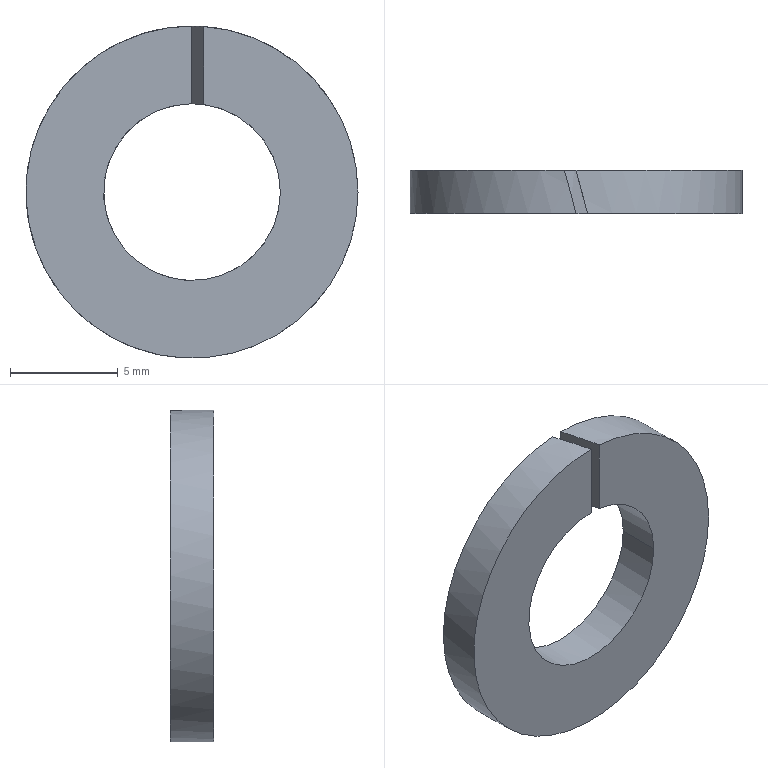Part | STEP file | ZZ24-M8 | 1 solid | 8 faces | box 15.4 x 2 x 15.4 mm | volume 263.048 mm3 | plane 4 | cylinder 4 | commonest cylinder face diameters 8.2 x2 15.4 x2
STEP:
#1=CARTESIAN_POINT('',(0.,0.,0.));
#2=DIRECTION('',(0.,0.,1.));
#3=DIRECTION('',(1.,0.,0.));
#4=AXIS2_PLACEMENT_3D('',#1,#2,#3);
#5=CARTESIAN_POINT('',(0.,0.,7.7));
#6=VERTEX_POINT('',#5);
#7=CARTESIAN_POINT('',(7.7,0.,0.));
#8=VERTEX_POINT('',#7);
#9=CARTESIAN_POINT('',(0.,0.,0.));
#10=DIRECTION('',(0.,-1.,0.));
#11=DIRECTION('',(0.,0.,1.));
#12=AXIS2_PLACEMENT_3D('',#9,#10,#11);
#13=CIRCLE('',#12,7.7);
#14=CARTESIAN_POINT('',(-16.334,0.,16.334));
#15=DIRECTION('',(0.,1.,0.));
#16=DIRECTION('',(1.,0.,0.));
#17=AXIS2_PLACEMENT_3D('',#14,#15,#16);
#18=PLANE('',#17);
#19=CARTESIAN_POINT('',(16.334,8.634));
#20=CARTESIAN_POINT('',(2.997,8.634));
#21=CARTESIAN_POINT('',(9.666,20.184));
#22=CARTESIAN_POINT('',(16.334,31.734));
#23=CARTESIAN_POINT('',(23.003,20.184));
#24=CARTESIAN_POINT('',(29.671,8.634));
#25=CARTESIAN_POINT('',(16.334,8.634));
#26=(BOUNDED_CURVE()B_SPLINE_CURVE(2,(#19,#20,#21,#22,#23,#24,#25),.UNSPECIFIED.,.T.,.F.)B_SPLINE_CURVE_WITH_KNOTS((1,2,2,2,2,1),(-2.094,0.,2.094,4.189,6.283,8.378),.UNSPECIFIED.)CURVE()GEOMETRIC_REPRESENTATION_ITEM()RATIONAL_B_SPLINE_CURVE((1.,0.5,1.,0.5,1.,0.5,1.))REPRESENTATION_ITEM(''));
#27=(GEOMETRIC_REPRESENTATION_CONTEXT(2)PARAMETRIC_REPRESENTATION_CONTEXT()REPRESENTATION_CONTEXT('',''));
#28=DEFINITIONAL_REPRESENTATION('',(#26),#27);
#29=PCURVE('',#18,#28);
#30=CARTESIAN_POINT('',(0.,1.,0.));
#31=DIRECTION('',(0.,1.,0.));
#32=DIRECTION('',(1.,0.,0.));
#33=AXIS2_PLACEMENT_3D('',#30,#31,#32);
#34=CYLINDRICAL_SURFACE('',#33,7.7);
#35=CARTESIAN_POINT('',(4.712,-1.));
#36=DIRECTION('',(-1.,0.));
#37=VECTOR('',#36,1.);
#38=LINE('',#35,#37);
#39=(GEOMETRIC_REPRESENTATION_CONTEXT(2)PARAMETRIC_REPRESENTATION_CONTEXT()REPRESENTATION_CONTEXT('',''));
#40=DEFINITIONAL_REPRESENTATION('',(#38),#39);
#41=PCURVE('',#34,#40);
#42=SURFACE_CURVE('',#13,(#29,#41),.PCURVE_S1.);
#43=EDGE_CURVE('',#6,#8,#42,.T.);
#44=ORIENTED_EDGE('',*,*,#43,.T.);
#45=CARTESIAN_POINT('',(0.5359,0.,7.681));
#46=VERTEX_POINT('',#45);
#47=CARTESIAN_POINT('',(0.,0.,0.));
#48=DIRECTION('',(0.,1.,0.));
#49=DIRECTION('',(0.0696,0.,0.9976));
#50=AXIS2_PLACEMENT_3D('',#47,#48,#49);
#51=CIRCLE('',#50,7.7);
#52=CARTESIAN_POINT('',(16.334,16.334));
#53=DIRECTION('',(0.0696,-0.9976));
#54=AXIS2_PLACEMENT_2D('',#52,#53);
#55=CIRCLE('',#54,7.7);
#56=(GEOMETRIC_REPRESENTATION_CONTEXT(2)PARAMETRIC_REPRESENTATION_CONTEXT()REPRESENTATION_CONTEXT('',''));
#57=DEFINITIONAL_REPRESENTATION('',(#55),#56);
#58=PCURVE('',#18,#57);
#59=CARTESIAN_POINT('',(0.,1.,0.));
#60=DIRECTION('',(0.,1.,0.));
#61=DIRECTION('',(1.,0.,0.));
#62=AXIS2_PLACEMENT_3D('',#59,#60,#61);
#63=CYLINDRICAL_SURFACE('',#62,7.7);
#64=CARTESIAN_POINT('',(4.782,-1.));
#65=DIRECTION('',(1.,0.));
#66=VECTOR('',#65,1.);
#67=LINE('',#64,#66);
#68=(GEOMETRIC_REPRESENTATION_CONTEXT(2)PARAMETRIC_REPRESENTATION_CONTEXT()REPRESENTATION_CONTEXT('',''));
#69=DEFINITIONAL_REPRESENTATION('',(#67),#68);
#70=PCURVE('',#63,#69);
#71=SURFACE_CURVE('',#51,(#58,#70),.PCURVE_S1.);
#72=EDGE_CURVE('',#46,#8,#71,.T.);
#73=ORIENTED_EDGE('',*,*,#72,.F.);
#74=CARTESIAN_POINT('',(0.5359,0.,4.065));
#75=VERTEX_POINT('',#74);
#76=CARTESIAN_POINT('',(0.5359,0.,7.681));
#77=DIRECTION('',(0.,0.,-1.));
#78=VECTOR('',#77,1.);
#79=LINE('',#76,#78);
#80=CARTESIAN_POINT('',(16.87,8.653));
#81=DIRECTION('',(0.,1.));
#82=VECTOR('',#81,1.);
#83=LINE('',#80,#82);
#84=(GEOMETRIC_REPRESENTATION_CONTEXT(2)PARAMETRIC_REPRESENTATION_CONTEXT()REPRESENTATION_CONTEXT('',''));
#85=DEFINITIONAL_REPRESENTATION('',(#83),#84);
#86=PCURVE('',#18,#85);
#87=CARTESIAN_POINT('',(1.08,-2.031,2.745));
#88=DIRECTION('',(0.9659,0.2588,0.));
#89=DIRECTION('',(-0.2588,0.9659,0.));
#90=AXIS2_PLACEMENT_3D('',#87,#88,#89);
#91=PLANE('',#90);
#92=CARTESIAN_POINT('',(2.102,4.937));
#93=DIRECTION('',(0.,-1.));
#94=VECTOR('',#93,1.);
#95=LINE('',#92,#94);
#96=(GEOMETRIC_REPRESENTATION_CONTEXT(2)PARAMETRIC_REPRESENTATION_CONTEXT()REPRESENTATION_CONTEXT('',''));
#97=DEFINITIONAL_REPRESENTATION('',(#95),#96);
#98=PCURVE('',#91,#97);
#99=SURFACE_CURVE('',#79,(#86,#98),.PCURVE_S1.);
#100=EDGE_CURVE('',#46,#75,#99,.T.);
#101=ORIENTED_EDGE('',*,*,#100,.T.);
#102=CARTESIAN_POINT('',(4.1,0.,0.));
#103=VERTEX_POINT('',#102);
#104=CARTESIAN_POINT('',(0.,0.,0.));
#105=DIRECTION('',(0.,-1.,0.));
#106=DIRECTION('',(1.,0.,0.));
#107=AXIS2_PLACEMENT_3D('',#104,#105,#106);
#108=CIRCLE('',#107,4.1);
#109=CARTESIAN_POINT('',(20.434,16.334));
#110=CARTESIAN_POINT('',(20.434,9.233));
#111=CARTESIAN_POINT('',(14.284,12.783));
#112=CARTESIAN_POINT('',(8.134,16.334));
#113=CARTESIAN_POINT('',(14.284,19.885));
#114=CARTESIAN_POINT('',(20.434,23.436));
#115=CARTESIAN_POINT('',(20.434,16.334));
#116=(BOUNDED_CURVE()B_SPLINE_CURVE(2,(#109,#110,#111,#112,#113,#114,#115),.UNSPECIFIED.,.T.,.F.)B_SPLINE_CURVE_WITH_KNOTS((1,2,2,2,2,1),(-2.094,0.,2.094,4.189,6.283,8.378),.UNSPECIFIED.)CURVE()GEOMETRIC_REPRESENTATION_ITEM()RATIONAL_B_SPLINE_CURVE((1.,0.5,1.,0.5,1.,0.5,1.))REPRESENTATION_ITEM(''));
#117=(GEOMETRIC_REPRESENTATION_CONTEXT(2)PARAMETRIC_REPRESENTATION_CONTEXT()REPRESENTATION_CONTEXT('',''));
#118=DEFINITIONAL_REPRESENTATION('',(#116),#117);
#119=PCURVE('',#18,#118);
#120=CARTESIAN_POINT('',(0.,1.,0.));
#121=DIRECTION('',(0.,1.,0.));
#122=DIRECTION('',(1.,0.,0.));
#123=AXIS2_PLACEMENT_3D('',#120,#121,#122);
#124=CYLINDRICAL_SURFACE('',#123,4.1);
#125=CARTESIAN_POINT('',(6.283,-1.));
#126=DIRECTION('',(-1.,0.));
#127=VECTOR('',#126,1.);
#128=LINE('',#125,#127);
#129=(GEOMETRIC_REPRESENTATION_CONTEXT(2)PARAMETRIC_REPRESENTATION_CONTEXT()REPRESENTATION_CONTEXT('',''));
#130=DEFINITIONAL_REPRESENTATION('',(#128),#129);
#131=PCURVE('',#124,#130);
#132=SURFACE_CURVE('',#108,(#119,#131),.PCURVE_S1.);
#133=EDGE_CURVE('',#103,#75,#132,.T.);
#134=ORIENTED_EDGE('',*,*,#133,.F.);
#135=CARTESIAN_POINT('',(0.,0.,4.1));
#136=VERTEX_POINT('',#135);
#137=CARTESIAN_POINT('',(0.,0.,0.));
#138=DIRECTION('',(0.,1.,0.));
#139=DIRECTION('',(1.,0.,0.));
#140=AXIS2_PLACEMENT_3D('',#137,#138,#139);
#141=CIRCLE('',#140,4.1);
#142=CARTESIAN_POINT('',(16.334,16.334));
#143=DIRECTION('',(1.,0.));
#144=AXIS2_PLACEMENT_2D('',#142,#143);
#145=CIRCLE('',#144,4.1);
#146=(GEOMETRIC_REPRESENTATION_CONTEXT(2)PARAMETRIC_REPRESENTATION_CONTEXT()REPRESENTATION_CONTEXT('',''));
#147=DEFINITIONAL_REPRESENTATION('',(#145),#146);
#148=PCURVE('',#18,#147);
#149=CARTESIAN_POINT('',(0.,1.,0.));
#150=DIRECTION('',(0.,1.,0.));
#151=DIRECTION('',(1.,0.,0.));
#152=AXIS2_PLACEMENT_3D('',#149,#150,#151);
#153=CYLINDRICAL_SURFACE('',#152,4.1);
#154=CARTESIAN_POINT('',(0.,-1.));
#155=DIRECTION('',(1.,0.));
#156=VECTOR('',#155,1.);
#157=LINE('',#154,#156);
#158=(GEOMETRIC_REPRESENTATION_CONTEXT(2)PARAMETRIC_REPRESENTATION_CONTEXT()REPRESENTATION_CONTEXT('',''));
#159=DEFINITIONAL_REPRESENTATION('',(#157),#158);
#160=PCURVE('',#153,#159);
#161=SURFACE_CURVE('',#141,(#148,#160),.PCURVE_S1.);
#162=EDGE_CURVE('',#103,#136,#161,.T.);
#163=ORIENTED_EDGE('',*,*,#162,.T.);
#164=CARTESIAN_POINT('',(0.,0.,7.7));
#165=DIRECTION('',(0.,0.,-1.));
#166=VECTOR('',#165,1.);
#167=LINE('',#164,#166);
#168=CARTESIAN_POINT('',(16.334,8.634));
#169=DIRECTION('',(0.,1.));
#170=VECTOR('',#169,1.);
#171=LINE('',#168,#170);
#172=(GEOMETRIC_REPRESENTATION_CONTEXT(2)PARAMETRIC_REPRESENTATION_CONTEXT()REPRESENTATION_CONTEXT('',''));
#173=DEFINITIONAL_REPRESENTATION('',(#171),#172);
#174=PCURVE('',#18,#173);
#175=CARTESIAN_POINT('',(-1.08,4.031,2.745));
#176=DIRECTION('',(-0.9659,-0.2588,0.));
#177=DIRECTION('',(0.2588,-0.9659,0.));
#178=AXIS2_PLACEMENT_3D('',#175,#176,#177);
#179=PLANE('',#178);
#180=CARTESIAN_POINT('',(4.173,4.955));
#181=DIRECTION('',(0.,-1.));
#182=VECTOR('',#181,1.);
#183=LINE('',#180,#182);
#184=(GEOMETRIC_REPRESENTATION_CONTEXT(2)PARAMETRIC_REPRESENTATION_CONTEXT()REPRESENTATION_CONTEXT('',''));
#185=DEFINITIONAL_REPRESENTATION('',(#183),#184);
#186=PCURVE('',#179,#185);
#187=SURFACE_CURVE('',#167,(#174,#186),.PCURVE_S1.);
#188=EDGE_CURVE('',#6,#136,#187,.T.);
#189=ORIENTED_EDGE('',*,*,#188,.F.);
#190=EDGE_LOOP('',(#44,#73,#101,#134,#163,#189));
#191=FACE_BOUND('',#190,.T.);
#192=ADVANCED_FACE('',(#191),#18,.F.);
#193=ORIENTED_EDGE('',*,*,#188,.T.);
#194=CARTESIAN_POINT('',(-0.5359,2.,4.065));
#195=VERTEX_POINT('',#194);
#196=CARTESIAN_POINT('',(-0.5359,2.,4.065));
#197=CARTESIAN_POINT('',(-0.3573,1.334,4.088));
#198=CARTESIAN_POINT('',(-0.1787,0.6668,4.1));
#199=CARTESIAN_POINT('',(0.,0.,4.1));
#200=B_SPLINE_CURVE_WITH_KNOTS('',3,(#196,#197,#198,#199),.UNSPECIFIED.,.F.,.F.,(4,4),(0.,1.),.PIECEWISE_BEZIER_KNOTS.);
#201=CARTESIAN_POINT('',(2.102,1.32));
#202=CARTESIAN_POINT('',(2.792,1.344));
#203=CARTESIAN_POINT('',(3.483,1.355));
#204=CARTESIAN_POINT('',(4.173,1.355));
#205=B_SPLINE_CURVE_WITH_KNOTS('',3,(#201,#202,#203,#204),.UNSPECIFIED.,.F.,.F.,(4,4),(0.,1.),.PIECEWISE_BEZIER_KNOTS.);
#206=(GEOMETRIC_REPRESENTATION_CONTEXT(2)PARAMETRIC_REPRESENTATION_CONTEXT()REPRESENTATION_CONTEXT('',''));
#207=DEFINITIONAL_REPRESENTATION('',(#205),#206);
#208=PCURVE('',#179,#207);
#209=CARTESIAN_POINT('',(4.581,1.));
#210=CARTESIAN_POINT('',(4.583,0.9697));
#211=CARTESIAN_POINT('',(4.587,0.9091));
#212=CARTESIAN_POINT('',(4.593,0.8182));
#213=CARTESIAN_POINT('',(4.599,0.7274));
#214=CARTESIAN_POINT('',(4.605,0.6365));
#215=CARTESIAN_POINT('',(4.611,0.5456));
#216=CARTESIAN_POINT('',(4.617,0.4547));
#217=CARTESIAN_POINT('',(4.623,0.3638));
#218=CARTESIAN_POINT('',(4.629,0.2729));
#219=CARTESIAN_POINT('',(4.635,0.182));
#220=CARTESIAN_POINT('',(4.641,0.09106));
#221=CARTESIAN_POINT('',(4.647,0.0001454));
#222=CARTESIAN_POINT('',(4.653,-0.09077));
#223=CARTESIAN_POINT('',(4.659,-0.1817));
#224=CARTESIAN_POINT('',(4.665,-0.2726));
#225=CARTESIAN_POINT('',(4.671,-0.3635));
#226=CARTESIAN_POINT('',(4.677,-0.4544));
#227=CARTESIAN_POINT('',(4.683,-0.5454));
#228=CARTESIAN_POINT('',(4.689,-0.6363));
#229=CARTESIAN_POINT('',(4.695,-0.7272));
#230=CARTESIAN_POINT('',(4.701,-0.8181));
#231=CARTESIAN_POINT('',(4.706,-0.9091));
#232=CARTESIAN_POINT('',(4.71,-0.9697));
#233=CARTESIAN_POINT('',(4.712,-1.));
#234=B_SPLINE_CURVE_WITH_KNOTS('',3,(#209,#210,#211,#212,#213,#214,#215,#216,#217,#218,#219,#220,#221,#222,#223,#224,#225,#226,#227,#228,#229,#230,#231,#232,#233),.UNSPECIFIED.,.F.,.F.,(4,1,1,1,1,1,1,1,1,1,1,1,1,1,1,1,1,1,1,1,1,1,4),(0.,0.04545,0.09091,0.1364,0.1818,0.2273,0.2727,0.3182,0.3636,0.4091,0.4545,0.5,0.5455,0.5909,0.6364,0.6818,0.7273,0.7727,0.8182,0.8636,0.9091,0.9545,1.),.QUASI_UNIFORM_KNOTS.);
#235=(GEOMETRIC_REPRESENTATION_CONTEXT(2)PARAMETRIC_REPRESENTATION_CONTEXT()REPRESENTATION_CONTEXT('',''));
#236=DEFINITIONAL_REPRESENTATION('',(#234),#235);
#237=PCURVE('',#153,#236);
#238=SURFACE_CURVE('',#200,(#208,#237),.PCURVE_S1.);
#239=EDGE_CURVE('',#195,#136,#238,.T.);
#240=ORIENTED_EDGE('',*,*,#239,.F.);
#241=CARTESIAN_POINT('',(-0.5359,2.,7.681));
#242=VERTEX_POINT('',#241);
#243=CARTESIAN_POINT('',(-0.5359,2.,7.681));
#244=DIRECTION('',(0.,0.,-1.));
#245=VECTOR('',#244,1.);
#246=LINE('',#243,#245);
#247=CARTESIAN_POINT('',(2.102,4.937));
#248=DIRECTION('',(0.,-1.));
#249=VECTOR('',#248,1.);
#250=LINE('',#247,#249);
#251=(GEOMETRIC_REPRESENTATION_CONTEXT(2)PARAMETRIC_REPRESENTATION_CONTEXT()REPRESENTATION_CONTEXT('',''));
#252=DEFINITIONAL_REPRESENTATION('',(#250),#251);
#253=PCURVE('',#179,#252);
#254=CARTESIAN_POINT('',(-16.777,2.,16.52));
#255=DIRECTION('',(0.,1.,0.));
#256=DIRECTION('',(1.,0.,0.));
#257=AXIS2_PLACEMENT_3D('',#254,#255,#256);
#258=PLANE('',#257);
#259=CARTESIAN_POINT('',(16.241,8.839));
#260=DIRECTION('',(0.,1.));
#261=VECTOR('',#260,1.);
#262=LINE('',#259,#261);
#263=(GEOMETRIC_REPRESENTATION_CONTEXT(2)PARAMETRIC_REPRESENTATION_CONTEXT()REPRESENTATION_CONTEXT('',''));
#264=DEFINITIONAL_REPRESENTATION('',(#262),#263);
#265=PCURVE('',#258,#264);
#266=SURFACE_CURVE('',#246,(#253,#265),.PCURVE_S1.);
#267=EDGE_CURVE('',#242,#195,#266,.T.);
#268=ORIENTED_EDGE('',*,*,#267,.F.);
#269=CARTESIAN_POINT('',(-0.0003089,0.001153,-106.985));
#270=DIRECTION('',(0.9659,0.2588,0.));
#271=DIRECTION('',(-0.00467,0.01743,0.9998));
#272=AXIS2_PLACEMENT_3D('',#269,#270,#271);
#273=CIRCLE('',#272,114.685);
#274=CARTESIAN_POINT('',(2.102,4.937));
#275=CARTESIAN_POINT('',(200.71,8.521));
#276=CARTESIAN_POINT('',(104.51,-165.271));
#277=CARTESIAN_POINT('',(8.31,-339.062));
#278=CARTESIAN_POINT('',(-94.097,-168.855));
#279=CARTESIAN_POINT('',(-196.505,1.352));
#280=CARTESIAN_POINT('',(2.102,4.937));
#281=(BOUNDED_CURVE()B_SPLINE_CURVE(2,(#274,#275,#276,#277,#278,#279,#280),.UNSPECIFIED.,.T.,.F.)B_SPLINE_CURVE_WITH_KNOTS((1,2,2,2,2,1),(-2.094,0.,2.094,4.189,6.283,8.378),.UNSPECIFIED.)CURVE()GEOMETRIC_REPRESENTATION_ITEM()RATIONAL_B_SPLINE_CURVE((1.,0.5,1.,0.5,1.,0.5,1.))REPRESENTATION_ITEM(''));
#282=(GEOMETRIC_REPRESENTATION_CONTEXT(2)PARAMETRIC_REPRESENTATION_CONTEXT()REPRESENTATION_CONTEXT('',''));
#283=DEFINITIONAL_REPRESENTATION('',(#281),#282);
#284=PCURVE('',#179,#283);
#285=CARTESIAN_POINT('',(4.643,1.));
#286=CARTESIAN_POINT('',(4.644,0.9697));
#287=CARTESIAN_POINT('',(4.646,0.9091));
#288=CARTESIAN_POINT('',(4.649,0.8182));
#289=CARTESIAN_POINT('',(4.652,0.7273));
#290=CARTESIAN_POINT('',(4.655,0.6364));
#291=CARTESIAN_POINT('',(4.659,0.5455));
#292=CARTESIAN_POINT('',(4.662,0.4546));
#293=CARTESIAN_POINT('',(4.665,0.3637));
#294=CARTESIAN_POINT('',(4.668,0.2728));
#295=CARTESIAN_POINT('',(4.671,0.1819));
#296=CARTESIAN_POINT('',(4.674,0.09095));
#297=CARTESIAN_POINT('',(4.678,0.00004082));
#298=CARTESIAN_POINT('',(4.681,-0.09087));
#299=CARTESIAN_POINT('',(4.684,-0.1818));
#300=CARTESIAN_POINT('',(4.687,-0.2727));
#301=CARTESIAN_POINT('',(4.69,-0.3636));
#302=CARTESIAN_POINT('',(4.693,-0.4545));
#303=CARTESIAN_POINT('',(4.697,-0.5454));
#304=CARTESIAN_POINT('',(4.7,-0.6363));
#305=CARTESIAN_POINT('',(4.703,-0.7273));
#306=CARTESIAN_POINT('',(4.706,-0.8182));
#307=CARTESIAN_POINT('',(4.709,-0.9091));
#308=CARTESIAN_POINT('',(4.711,-0.9697));
#309=CARTESIAN_POINT('',(4.712,-1.));
#310=B_SPLINE_CURVE_WITH_KNOTS('',3,(#285,#286,#287,#288,#289,#290,#291,#292,#293,#294,#295,#296,#297,#298,#299,#300,#301,#302,#303,#304,#305,#306,#307,#308,#309),.UNSPECIFIED.,.F.,.F.,(4,1,1,1,1,1,1,1,1,1,1,1,1,1,1,1,1,1,1,1,1,1,4),(0.,0.0008207,0.001641,0.002462,0.003283,0.004103,0.004924,0.005745,0.006566,0.007386,0.008207,0.009028,0.009848,0.01067,0.01149,0.01231,0.01313,0.01395,0.01477,0.01559,0.01641,0.01723,0.01806),.QUASI_UNIFORM_KNOTS.);
#311=(GEOMETRIC_REPRESENTATION_CONTEXT(2)PARAMETRIC_REPRESENTATION_CONTEXT()REPRESENTATION_CONTEXT('',''));
#312=DEFINITIONAL_REPRESENTATION('',(#310),#311);
#313=PCURVE('',#34,#312);
#314=SURFACE_CURVE('',#273,(#284,#313),.PCURVE_S1.);
#315=EDGE_CURVE('',#242,#6,#314,.T.);
#316=ORIENTED_EDGE('',*,*,#315,.T.);
#317=EDGE_LOOP('',(#193,#240,#268,#316));
#318=FACE_BOUND('',#317,.T.);
#319=ADVANCED_FACE('',(#318),#179,.F.);
#320=CARTESIAN_POINT('',(7.7,2.,0.));
#321=VERTEX_POINT('',#320);
#322=CARTESIAN_POINT('',(7.7,0.,0.));
#323=DIRECTION('',(0.,1.,0.));
#324=VECTOR('',#323,1.);
#325=LINE('',#322,#324);
#326=CARTESIAN_POINT('',(0.,-1.));
#327=DIRECTION('',(0.,1.));
#328=VECTOR('',#327,1.);
#329=LINE('',#326,#328);
#330=(GEOMETRIC_REPRESENTATION_CONTEXT(2)PARAMETRIC_REPRESENTATION_CONTEXT()REPRESENTATION_CONTEXT('',''));
#331=DEFINITIONAL_REPRESENTATION('',(#329),#330);
#332=PCURVE('',#34,#331);
#333=CARTESIAN_POINT('',(6.283,-1.));
#334=DIRECTION('',(0.,1.));
#335=VECTOR('',#334,1.);
#336=LINE('',#333,#335);
#337=(GEOMETRIC_REPRESENTATION_CONTEXT(2)PARAMETRIC_REPRESENTATION_CONTEXT()REPRESENTATION_CONTEXT('',''));
#338=DEFINITIONAL_REPRESENTATION('',(#336),#337);
#339=PCURVE('',#63,#338);
#340=SURFACE_CURVE('',#325,(#332,#339),.PCURVE_S1.);
#341=EDGE_CURVE('',#8,#321,#340,.T.);
#342=ORIENTED_EDGE('',*,*,#341,.F.);
#343=ORIENTED_EDGE('',*,*,#43,.F.);
#344=ORIENTED_EDGE('',*,*,#315,.F.);
#345=CARTESIAN_POINT('',(0.,2.,0.));
#346=DIRECTION('',(0.,1.,0.));
#347=DIRECTION('',(1.,0.,0.));
#348=AXIS2_PLACEMENT_3D('',#345,#346,#347);
#349=CIRCLE('',#348,7.7);
#350=CARTESIAN_POINT('',(0.,1.));
#351=DIRECTION('',(1.,0.));
#352=VECTOR('',#351,1.);
#353=LINE('',#350,#352);
#354=(GEOMETRIC_REPRESENTATION_CONTEXT(2)PARAMETRIC_REPRESENTATION_CONTEXT()REPRESENTATION_CONTEXT('',''));
#355=DEFINITIONAL_REPRESENTATION('',(#353),#354);
#356=PCURVE('',#34,#355);
#357=CARTESIAN_POINT('',(16.777,16.52));
#358=DIRECTION('',(1.,0.));
#359=AXIS2_PLACEMENT_2D('',#357,#358);
#360=CIRCLE('',#359,7.7);
#361=(GEOMETRIC_REPRESENTATION_CONTEXT(2)PARAMETRIC_REPRESENTATION_CONTEXT()REPRESENTATION_CONTEXT('',''));
#362=DEFINITIONAL_REPRESENTATION('',(#360),#361);
#363=PCURVE('',#258,#362);
#364=SURFACE_CURVE('',#349,(#356,#363),.PCURVE_S1.);
#365=EDGE_CURVE('',#321,#242,#364,.T.);
#366=ORIENTED_EDGE('',*,*,#365,.F.);
#367=EDGE_LOOP('',(#342,#343,#344,#366));
#368=FACE_BOUND('',#367,.T.);
#369=ADVANCED_FACE('',(#368),#34,.T.);
#370=CARTESIAN_POINT('',(4.1,2.,0.));
#371=VERTEX_POINT('',#370);
#372=CARTESIAN_POINT('',(0.,2.,0.));
#373=DIRECTION('',(0.,-1.,0.));
#374=DIRECTION('',(-0.1307,0.,0.9914));
#375=AXIS2_PLACEMENT_3D('',#372,#373,#374);
#376=CIRCLE('',#375,4.1);
#377=CARTESIAN_POINT('',(16.241,12.456));
#378=CARTESIAN_POINT('',(9.201,13.384));
#379=CARTESIAN_POINT('',(13.525,19.017));
#380=CARTESIAN_POINT('',(17.849,24.65));
#381=CARTESIAN_POINT('',(20.565,18.089));
#382=CARTESIAN_POINT('',(23.282,11.527));
#383=CARTESIAN_POINT('',(16.241,12.456));
#384=(BOUNDED_CURVE()B_SPLINE_CURVE(2,(#377,#378,#379,#380,#381,#382,#383),.UNSPECIFIED.,.T.,.F.)B_SPLINE_CURVE_WITH_KNOTS((1,2,2,2,2,1),(-2.094,0.,2.094,4.189,6.283,8.378),.UNSPECIFIED.)CURVE()GEOMETRIC_REPRESENTATION_ITEM()RATIONAL_B_SPLINE_CURVE((1.,0.5,1.,0.5,1.,0.5,1.))REPRESENTATION_ITEM(''));
#385=(GEOMETRIC_REPRESENTATION_CONTEXT(2)PARAMETRIC_REPRESENTATION_CONTEXT()REPRESENTATION_CONTEXT('',''));
#386=DEFINITIONAL_REPRESENTATION('',(#384),#385);
#387=PCURVE('',#258,#386);
#388=CARTESIAN_POINT('',(4.581,1.));
#389=DIRECTION('',(-1.,0.));
#390=VECTOR('',#389,1.);
#391=LINE('',#388,#390);
#392=(GEOMETRIC_REPRESENTATION_CONTEXT(2)PARAMETRIC_REPRESENTATION_CONTEXT()REPRESENTATION_CONTEXT('',''));
#393=DEFINITIONAL_REPRESENTATION('',(#391),#392);
#394=PCURVE('',#153,#393);
#395=SURFACE_CURVE('',#376,(#387,#394),.PCURVE_S1.);
#396=EDGE_CURVE('',#195,#371,#395,.T.);
#397=ORIENTED_EDGE('',*,*,#396,.T.);
#398=CARTESIAN_POINT('',(0.,2.,4.1));
#399=VERTEX_POINT('',#398);
#400=CARTESIAN_POINT('',(0.,2.,0.));
#401=DIRECTION('',(0.,-1.,0.));
#402=DIRECTION('',(1.,0.,0.));
#403=AXIS2_PLACEMENT_3D('',#400,#401,#402);
#404=CIRCLE('',#403,4.1);
#405=CARTESIAN_POINT('',(20.877,16.52));
#406=CARTESIAN_POINT('',(20.877,9.419));
#407=CARTESIAN_POINT('',(14.727,12.97));
#408=CARTESIAN_POINT('',(8.577,16.52));
#409=CARTESIAN_POINT('',(14.727,20.071));
#410=CARTESIAN_POINT('',(20.877,23.622));
#411=CARTESIAN_POINT('',(20.877,16.52));
#412=(BOUNDED_CURVE()B_SPLINE_CURVE(2,(#405,#406,#407,#408,#409,#410,#411),.UNSPECIFIED.,.T.,.F.)B_SPLINE_CURVE_WITH_KNOTS((1,2,2,2,2,1),(-2.094,0.,2.094,4.189,6.283,8.378),.UNSPECIFIED.)CURVE()GEOMETRIC_REPRESENTATION_ITEM()RATIONAL_B_SPLINE_CURVE((1.,0.5,1.,0.5,1.,0.5,1.))REPRESENTATION_ITEM(''));
#413=(GEOMETRIC_REPRESENTATION_CONTEXT(2)PARAMETRIC_REPRESENTATION_CONTEXT()REPRESENTATION_CONTEXT('',''));
#414=DEFINITIONAL_REPRESENTATION('',(#412),#413);
#415=PCURVE('',#258,#414);
#416=CARTESIAN_POINT('',(6.283,1.));
#417=DIRECTION('',(-1.,0.));
#418=VECTOR('',#417,1.);
#419=LINE('',#416,#418);
#420=(GEOMETRIC_REPRESENTATION_CONTEXT(2)PARAMETRIC_REPRESENTATION_CONTEXT()REPRESENTATION_CONTEXT('',''));
#421=DEFINITIONAL_REPRESENTATION('',(#419),#420);
#422=PCURVE('',#124,#421);
#423=SURFACE_CURVE('',#404,(#415,#422),.PCURVE_S1.);
#424=EDGE_CURVE('',#371,#399,#423,.T.);
#425=ORIENTED_EDGE('',*,*,#424,.T.);
#426=CARTESIAN_POINT('',(0.,2.,7.7));
#427=VERTEX_POINT('',#426);
#428=CARTESIAN_POINT('',(0.,2.,7.7));
#429=DIRECTION('',(0.,0.,-1.));
#430=VECTOR('',#429,1.);
#431=LINE('',#428,#430);
#432=CARTESIAN_POINT('',(16.777,8.82));
#433=DIRECTION('',(0.,1.));
#434=VECTOR('',#433,1.);
#435=LINE('',#432,#434);
#436=(GEOMETRIC_REPRESENTATION_CONTEXT(2)PARAMETRIC_REPRESENTATION_CONTEXT()REPRESENTATION_CONTEXT('',''));
#437=DEFINITIONAL_REPRESENTATION('',(#435),#436);
#438=PCURVE('',#258,#437);
#439=CARTESIAN_POINT('',(4.173,4.955));
#440=DIRECTION('',(0.,-1.));
#441=VECTOR('',#440,1.);
#442=LINE('',#439,#441);
#443=(GEOMETRIC_REPRESENTATION_CONTEXT(2)PARAMETRIC_REPRESENTATION_CONTEXT()REPRESENTATION_CONTEXT('',''));
#444=DEFINITIONAL_REPRESENTATION('',(#442),#443);
#445=PCURVE('',#91,#444);
#446=SURFACE_CURVE('',#431,(#438,#445),.PCURVE_S1.);
#447=EDGE_CURVE('',#427,#399,#446,.T.);
#448=ORIENTED_EDGE('',*,*,#447,.F.);
#449=CARTESIAN_POINT('',(0.,2.,0.));
#450=DIRECTION('',(0.,1.,0.));
#451=DIRECTION('',(0.,0.,1.));
#452=AXIS2_PLACEMENT_3D('',#449,#450,#451);
#453=CIRCLE('',#452,7.7);
#454=CARTESIAN_POINT('',(16.777,16.52));
#455=DIRECTION('',(0.,-1.));
#456=AXIS2_PLACEMENT_2D('',#454,#455);
#457=CIRCLE('',#456,7.7);
#458=(GEOMETRIC_REPRESENTATION_CONTEXT(2)PARAMETRIC_REPRESENTATION_CONTEXT()REPRESENTATION_CONTEXT('',''));
#459=DEFINITIONAL_REPRESENTATION('',(#457),#458);
#460=PCURVE('',#258,#459);
#461=CARTESIAN_POINT('',(4.712,1.));
#462=DIRECTION('',(1.,0.));
#463=VECTOR('',#462,1.);
#464=LINE('',#461,#463);
#465=(GEOMETRIC_REPRESENTATION_CONTEXT(2)PARAMETRIC_REPRESENTATION_CONTEXT()REPRESENTATION_CONTEXT('',''));
#466=DEFINITIONAL_REPRESENTATION('',(#464),#465);
#467=PCURVE('',#63,#466);
#468=SURFACE_CURVE('',#453,(#460,#467),.PCURVE_S1.);
#469=EDGE_CURVE('',#427,#321,#468,.T.);
#470=ORIENTED_EDGE('',*,*,#469,.T.);
#471=ORIENTED_EDGE('',*,*,#365,.T.);
#472=ORIENTED_EDGE('',*,*,#267,.T.);
#473=EDGE_LOOP('',(#397,#425,#448,#470,#471,#472));
#474=FACE_BOUND('',#473,.T.);
#475=ADVANCED_FACE('',(#474),#258,.T.);
#476=ORIENTED_EDGE('',*,*,#72,.T.);
#477=ORIENTED_EDGE('',*,*,#341,.T.);
#478=ORIENTED_EDGE('',*,*,#469,.F.);
#479=CARTESIAN_POINT('',(0.0003089,1.999,-106.985));
#480=DIRECTION('',(0.9659,0.2588,0.));
#481=DIRECTION('',(-0.000002693,0.00001005,1.));
#482=AXIS2_PLACEMENT_3D('',#479,#480,#481);
#483=CIRCLE('',#482,114.685);
#484=CARTESIAN_POINT('',(4.712,1.));
#485=CARTESIAN_POINT('',(4.713,0.9697));
#486=CARTESIAN_POINT('',(4.716,0.9091));
#487=CARTESIAN_POINT('',(4.719,0.8182));
#488=CARTESIAN_POINT('',(4.722,0.7273));
#489=CARTESIAN_POINT('',(4.725,0.6363));
#490=CARTESIAN_POINT('',(4.728,0.5454));
#491=CARTESIAN_POINT('',(4.731,0.4545));
#492=CARTESIAN_POINT('',(4.735,0.3636));
#493=CARTESIAN_POINT('',(4.738,0.2727));
#494=CARTESIAN_POINT('',(4.741,0.1818));
#495=CARTESIAN_POINT('',(4.744,0.09087));
#496=CARTESIAN_POINT('',(4.747,-0.00004082));
#497=CARTESIAN_POINT('',(4.75,-0.09095));
#498=CARTESIAN_POINT('',(4.754,-0.1819));
#499=CARTESIAN_POINT('',(4.757,-0.2728));
#500=CARTESIAN_POINT('',(4.76,-0.3637));
#501=CARTESIAN_POINT('',(4.763,-0.4546));
#502=CARTESIAN_POINT('',(4.766,-0.5455));
#503=CARTESIAN_POINT('',(4.769,-0.6364));
#504=CARTESIAN_POINT('',(4.773,-0.7273));
#505=CARTESIAN_POINT('',(4.776,-0.8182));
#506=CARTESIAN_POINT('',(4.779,-0.9091));
#507=CARTESIAN_POINT('',(4.781,-0.9697));
#508=CARTESIAN_POINT('',(4.782,-1.));
#509=B_SPLINE_CURVE_WITH_KNOTS('',3,(#484,#485,#486,#487,#488,#489,#490,#491,#492,#493,#494,#495,#496,#497,#498,#499,#500,#501,#502,#503,#504,#505,#506,#507,#508),.UNSPECIFIED.,.F.,.F.,(4,1,1,1,1,1,1,1,1,1,1,1,1,1,1,1,1,1,1,1,1,1,4),(0.,0.0008207,0.001641,0.002462,0.003283,0.004103,0.004924,0.005745,0.006566,0.007386,0.008207,0.009028,0.009848,0.01067,0.01149,0.01231,0.01313,0.01395,0.01477,0.01559,0.01641,0.01723,0.01806),.QUASI_UNIFORM_KNOTS.);
#510=(GEOMETRIC_REPRESENTATION_CONTEXT(2)PARAMETRIC_REPRESENTATION_CONTEXT()REPRESENTATION_CONTEXT('',''));
#511=DEFINITIONAL_REPRESENTATION('',(#509),#510);
#512=PCURVE('',#63,#511);
#513=CARTESIAN_POINT('',(4.172,-109.73));
#514=DIRECTION('',(0.00001041,1.));
#515=AXIS2_PLACEMENT_2D('',#513,#514);
#516=CIRCLE('',#515,114.685);
#517=(GEOMETRIC_REPRESENTATION_CONTEXT(2)PARAMETRIC_REPRESENTATION_CONTEXT()REPRESENTATION_CONTEXT('',''));
#518=DEFINITIONAL_REPRESENTATION('',(#516),#517);
#519=PCURVE('',#91,#518);
#520=SURFACE_CURVE('',#483,(#512,#519),.PCURVE_S1.);
#521=EDGE_CURVE('',#427,#46,#520,.T.);
#522=ORIENTED_EDGE('',*,*,#521,.T.);
#523=EDGE_LOOP('',(#476,#477,#478,#522));
#524=FACE_BOUND('',#523,.T.);
#525=ADVANCED_FACE('',(#524),#63,.T.);
#526=ORIENTED_EDGE('',*,*,#100,.F.);
#527=ORIENTED_EDGE('',*,*,#521,.F.);
#528=ORIENTED_EDGE('',*,*,#447,.T.);
#529=CARTESIAN_POINT('',(0.,2.,4.1));
#530=CARTESIAN_POINT('',(0.1787,1.333,4.1));
#531=CARTESIAN_POINT('',(0.3573,0.6664,4.088));
#532=CARTESIAN_POINT('',(0.5359,0.,4.065));
#533=B_SPLINE_CURVE_WITH_KNOTS('',3,(#529,#530,#531,#532),.UNSPECIFIED.,.F.,.F.,(4,4),(0.,1.),.PIECEWISE_BEZIER_KNOTS.);
#534=CARTESIAN_POINT('',(4.173,1.355));
#535=CARTESIAN_POINT('',(3.483,1.355));
#536=CARTESIAN_POINT('',(2.792,1.344));
#537=CARTESIAN_POINT('',(2.102,1.32));
#538=B_SPLINE_CURVE_WITH_KNOTS('',3,(#534,#535,#536,#537),.UNSPECIFIED.,.F.,.F.,(4,4),(0.,1.),.PIECEWISE_BEZIER_KNOTS.);
#539=(GEOMETRIC_REPRESENTATION_CONTEXT(2)PARAMETRIC_REPRESENTATION_CONTEXT()REPRESENTATION_CONTEXT('',''));
#540=DEFINITIONAL_REPRESENTATION('',(#538),#539);
#541=PCURVE('',#91,#540);
#542=CARTESIAN_POINT('',(4.712,1.));
#543=CARTESIAN_POINT('',(4.714,0.9697));
#544=CARTESIAN_POINT('',(4.718,0.9091));
#545=CARTESIAN_POINT('',(4.724,0.8181));
#546=CARTESIAN_POINT('',(4.73,0.7272));
#547=CARTESIAN_POINT('',(4.736,0.6363));
#548=CARTESIAN_POINT('',(4.742,0.5454));
#549=CARTESIAN_POINT('',(4.748,0.4544));
#550=CARTESIAN_POINT('',(4.754,0.3635));
#551=CARTESIAN_POINT('',(4.76,0.2726));
#552=CARTESIAN_POINT('',(4.766,0.1817));
#553=CARTESIAN_POINT('',(4.772,0.09077));
#554=CARTESIAN_POINT('',(4.778,-0.0001454));
#555=CARTESIAN_POINT('',(4.784,-0.09106));
#556=CARTESIAN_POINT('',(4.79,-0.182));
#557=CARTESIAN_POINT('',(4.796,-0.2729));
#558=CARTESIAN_POINT('',(4.802,-0.3638));
#559=CARTESIAN_POINT('',(4.808,-0.4547));
#560=CARTESIAN_POINT('',(4.814,-0.5456));
#561=CARTESIAN_POINT('',(4.82,-0.6365));
#562=CARTESIAN_POINT('',(4.826,-0.7274));
#563=CARTESIAN_POINT('',(4.831,-0.8182));
#564=CARTESIAN_POINT('',(4.837,-0.9091));
#565=CARTESIAN_POINT('',(4.841,-0.9697));
#566=CARTESIAN_POINT('',(4.843,-1.));
#567=B_SPLINE_CURVE_WITH_KNOTS('',3,(#542,#543,#544,#545,#546,#547,#548,#549,#550,#551,#552,#553,#554,#555,#556,#557,#558,#559,#560,#561,#562,#563,#564,#565,#566),.UNSPECIFIED.,.F.,.F.,(4,1,1,1,1,1,1,1,1,1,1,1,1,1,1,1,1,1,1,1,1,1,4),(0.,0.04545,0.09091,0.1364,0.1818,0.2273,0.2727,0.3182,0.3636,0.4091,0.4545,0.5,0.5455,0.5909,0.6364,0.6818,0.7273,0.7727,0.8182,0.8636,0.9091,0.9545,1.),.QUASI_UNIFORM_KNOTS.);
#568=(GEOMETRIC_REPRESENTATION_CONTEXT(2)PARAMETRIC_REPRESENTATION_CONTEXT()REPRESENTATION_CONTEXT('',''));
#569=DEFINITIONAL_REPRESENTATION('',(#567),#568);
#570=PCURVE('',#124,#569);
#571=SURFACE_CURVE('',#533,(#541,#570),.PCURVE_S1.);
#572=EDGE_CURVE('',#399,#75,#571,.T.);
#573=ORIENTED_EDGE('',*,*,#572,.T.);
#574=EDGE_LOOP('',(#526,#527,#528,#573));
#575=FACE_BOUND('',#574,.T.);
#576=ADVANCED_FACE('',(#575),#91,.F.);
#577=ORIENTED_EDGE('',*,*,#572,.T.);
#578=ORIENTED_EDGE('',*,*,#133,.F.);
#579=CARTESIAN_POINT('',(4.1,0.,0.));
#580=DIRECTION('',(0.,1.,0.));
#581=VECTOR('',#580,1.);
#582=LINE('',#579,#581);
#583=CARTESIAN_POINT('',(6.283,-1.));
#584=DIRECTION('',(0.,1.));
#585=VECTOR('',#584,1.);
#586=LINE('',#583,#585);
#587=(GEOMETRIC_REPRESENTATION_CONTEXT(2)PARAMETRIC_REPRESENTATION_CONTEXT()REPRESENTATION_CONTEXT('',''));
#588=DEFINITIONAL_REPRESENTATION('',(#586),#587);
#589=PCURVE('',#124,#588);
#590=CARTESIAN_POINT('',(0.,-1.));
#591=DIRECTION('',(0.,1.));
#592=VECTOR('',#591,1.);
#593=LINE('',#590,#592);
#594=(GEOMETRIC_REPRESENTATION_CONTEXT(2)PARAMETRIC_REPRESENTATION_CONTEXT()REPRESENTATION_CONTEXT('',''));
#595=DEFINITIONAL_REPRESENTATION('',(#593),#594);
#596=PCURVE('',#153,#595);
#597=SURFACE_CURVE('',#582,(#589,#596),.PCURVE_S1.);
#598=EDGE_CURVE('',#103,#371,#597,.T.);
#599=ORIENTED_EDGE('',*,*,#598,.T.);
#600=ORIENTED_EDGE('',*,*,#424,.T.);
#601=EDGE_LOOP('',(#577,#578,#599,#600));
#602=FACE_BOUND('',#601,.F.);
#603=ADVANCED_FACE('',(#602),#124,.F.);
#604=ORIENTED_EDGE('',*,*,#162,.T.);
#605=ORIENTED_EDGE('',*,*,#239,.F.);
#606=ORIENTED_EDGE('',*,*,#396,.T.);
#607=ORIENTED_EDGE('',*,*,#598,.F.);
#608=EDGE_LOOP('',(#604,#605,#606,#607));
#609=FACE_BOUND('',#608,.F.);
#610=ADVANCED_FACE('',(#609),#153,.F.);
#611=CLOSED_SHELL('',(#192,#319,#369,#475,#525,#576,#603,#610));
#612=MANIFOLD_SOLID_BREP('',#611);
#613=(LENGTH_UNIT()NAMED_UNIT(*)SI_UNIT(.MILLI.,.METRE.));
#614=UNCERTAINTY_MEASURE_WITH_UNIT(LENGTH_MEASURE(0.000002),#613,'','');
#615=(NAMED_UNIT(*)PLANE_ANGLE_UNIT()SI_UNIT($,.RADIAN.));
#616=(NAMED_UNIT(*)SI_UNIT($,.STERADIAN.)SOLID_ANGLE_UNIT());
#617=(GEOMETRIC_REPRESENTATION_CONTEXT(3)GLOBAL_UNCERTAINTY_ASSIGNED_CONTEXT((#614))GLOBAL_UNIT_ASSIGNED_CONTEXT((#613,#615,#616))REPRESENTATION_CONTEXT('',''));
#618=ADVANCED_BREP_SHAPE_REPRESENTATION('',(#4,#612),#617);